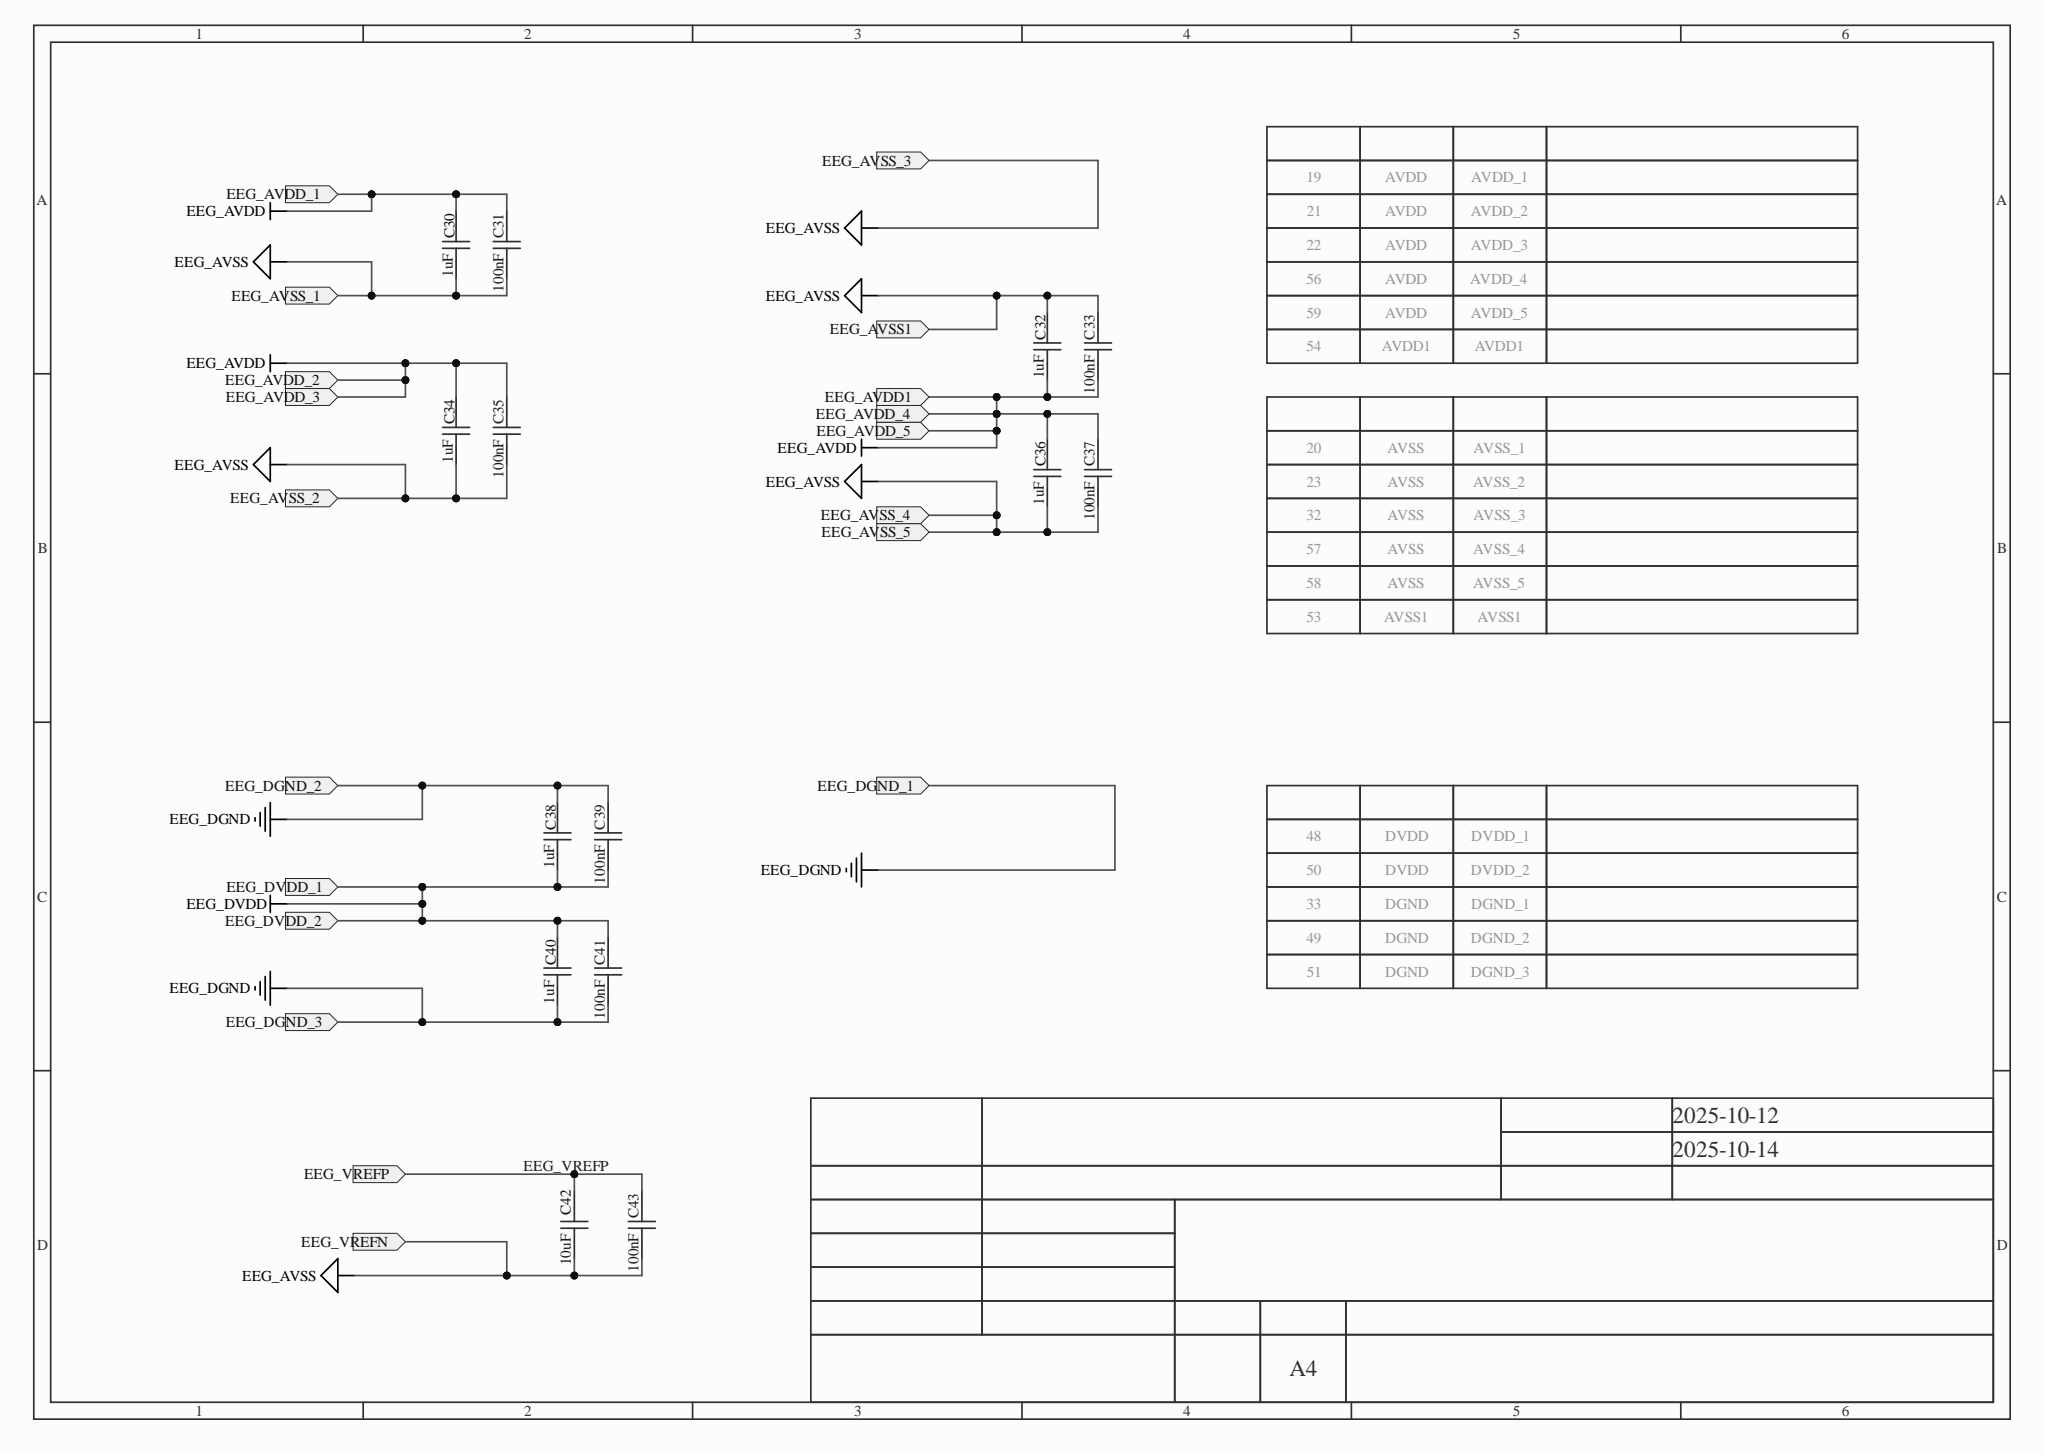Circuit board | Altium Designer | 212 parts | 123 nets | one sheet of the schematic
Parts on this sheet (reference | value | footprint):
C30 | 1uF | C0402
C31 | 100nF | C0402
C32 | 1uF | C0402
C33 | 100nF | C0402
C34 | 1uF | C0402
C35 | 100nF | C0402
C36 | 1uF | C0402
C37 | 100nF | C0402
C38 | 1uF | C0402
C39 | 100nF | C0402
C40 | 1uF | C0402
C41 | 100nF | C0402
C42 | 10uF | C0603
C43 | 100nF | C0402
Nets of these parts (net: part-pin ...):
EEG_VREFP: C42-2 C43-2
EEG_DVDD_1: C38-1 C39-1 C40-2 C41-2
EEG_DGND_1: C38-2 C39-2 C40-1 C41-1
EEG_AVSS1: C30-1 C31-1 C32-2 C33-2 C34-1 C35-1 C36-1 C37-1 C42-1 C43-1
EEG_AVDD1: C30-2 C31-2 C32-1 C33-1 C34-2 C35-2 C36-2 C37-2